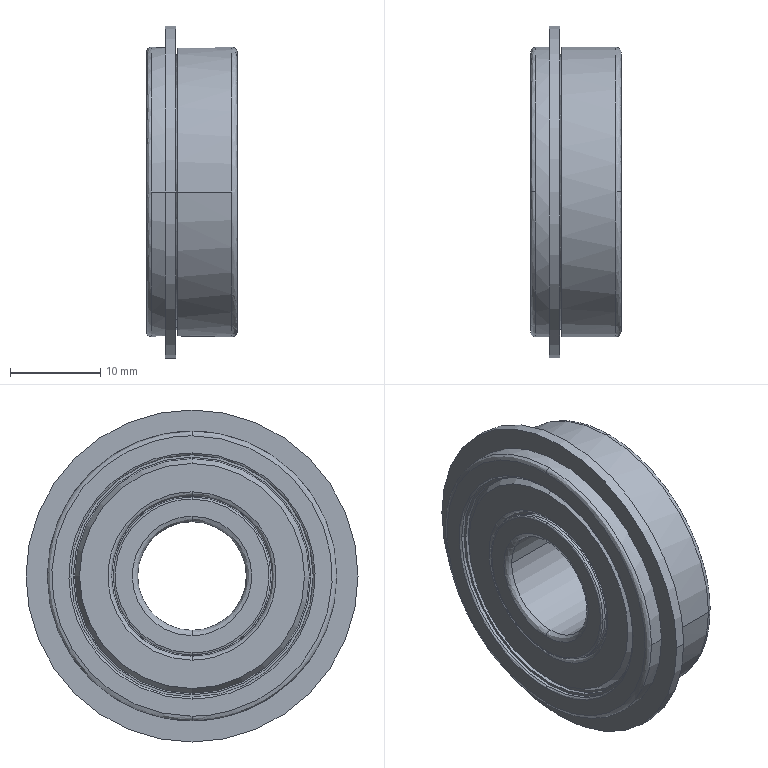Part | STEP file | Bearing B6201ZZNR_MISUMI | 1 solid | 115 faces | box 10 x 36.7 x 36.7 mm | volume 5407 mm3 | cylinder 42 | spline 40 | plane 25 | cone 8 | commonest cylinder face diameters 26.8 x8 16.6 x4 17.4 x4 17.8 x4 18.6 x4 26.27 x4